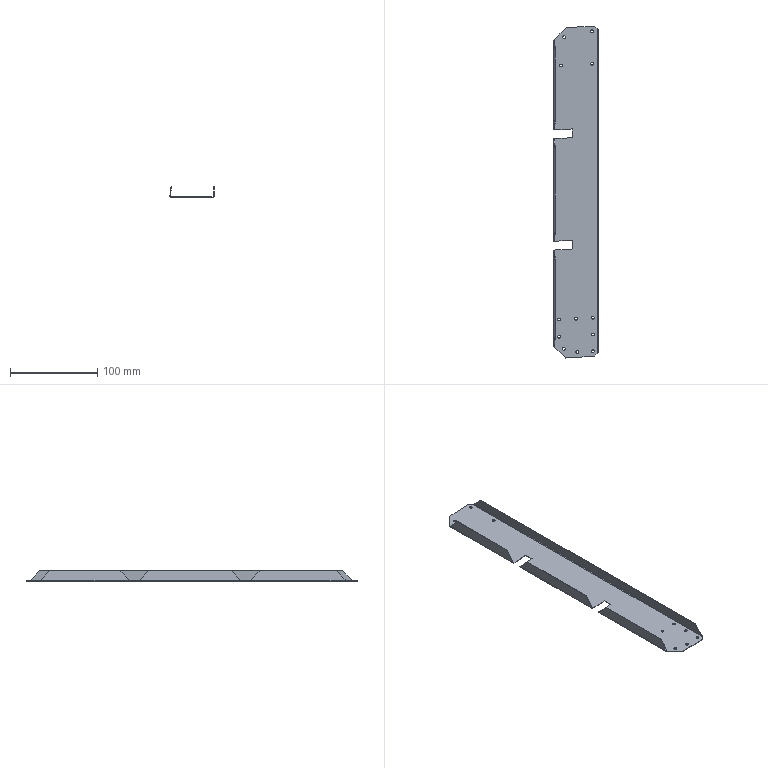Part | SolidWorks | features BaseBody 1 | 1 solid | 78 faces | box 50.77 x 379.903 x 11.911 mm | volume 12859 mm3 | plane 34 | cylinder 32 | spline 12 | commonest cylinder face diameters 3.2 x24 1 x4 2 x4